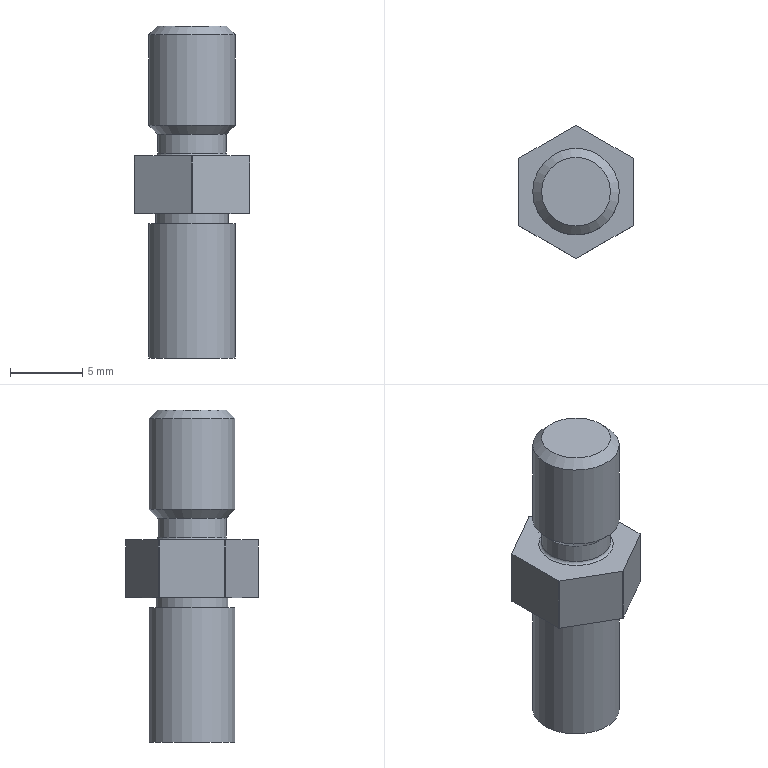Part | NX | features BREP 1 | 1 solid | 27 faces | box 8 x 9.2 x 23 mm | volume 695.67 mm3 | plane 11 | cylinder 11 | cone 4 | torus 1 | commonest cylinder face diameters 9.2 x6 6 x2 2.459 x1 4.773 x1 5 x1
STEP:
#1=CARTESIAN_POINT('',(-0.03277,4.6,-9.));
#2=VERTEX_POINT('',#1);
#3=CARTESIAN_POINT('',(-0.03277,4.6,-13.));
#4=VERTEX_POINT('',#3);
#5=CARTESIAN_POINT('',(-0.03277,4.6,-23.));
#6=DIRECTION('',(0.,0.,-1.));
#7=VECTOR('',#6,1000.);
#8=LINE('',#5,#7);
#9=EDGE_CURVE('',#2,#4,#8,.T.);
#10=ORIENTED_EDGE('',*,*,#9,.T.);
#11=CARTESIAN_POINT('',(-3.967,2.328,-13.));
#12=VERTEX_POINT('',#11);
#13=CARTESIAN_POINT('',(0.,4.619,-13.));
#14=DIRECTION('',(-0.866,-0.5,0.));
#15=VECTOR('',#14,1000.);
#16=LINE('',#13,#15);
#17=EDGE_CURVE('',#4,#12,#16,.T.);
#18=ORIENTED_EDGE('',*,*,#17,.T.);
#19=CARTESIAN_POINT('',(-3.967,2.328,-9.));
#20=VERTEX_POINT('',#19);
#21=CARTESIAN_POINT('',(-3.967,2.328,-23.));
#22=DIRECTION('',(0.,0.,-1.));
#23=VECTOR('',#22,1000.);
#24=LINE('',#21,#23);
#25=EDGE_CURVE('',#20,#12,#24,.T.);
#26=ORIENTED_EDGE('',*,*,#25,.F.);
#27=CARTESIAN_POINT('',(0.,4.619,-9.));
#28=DIRECTION('',(-0.866,-0.5,0.));
#29=VECTOR('',#28,1000.);
#30=LINE('',#27,#29);
#31=EDGE_CURVE('',#2,#20,#30,.T.);
#32=ORIENTED_EDGE('',*,*,#31,.F.);
#33=EDGE_LOOP('',(#10,#18,#26,#32));
#34=FACE_BOUND('',#33,.T.);
#35=CARTESIAN_POINT('',(0.,4.619,-13.));
#36=DIRECTION('',(-0.5,0.866,0.));
#37=DIRECTION('',(-0.866,-0.5,0.));
#38=AXIS2_PLACEMENT_3D('',#35,#36,#37);
#39=PLANE('',#38);
#40=ADVANCED_FACE('',(#34),#39,.T.);
#41=CARTESIAN_POINT('',(3.967,2.328,-9.));
#42=VERTEX_POINT('',#41);
#43=CARTESIAN_POINT('',(3.967,2.328,-13.));
#44=VERTEX_POINT('',#43);
#45=CARTESIAN_POINT('',(3.967,2.328,-23.));
#46=DIRECTION('',(0.,0.,-1.));
#47=VECTOR('',#46,1000.);
#48=LINE('',#45,#47);
#49=EDGE_CURVE('',#42,#44,#48,.T.);
#50=ORIENTED_EDGE('',*,*,#49,.T.);
#51=CARTESIAN_POINT('',(0.03277,4.6,-13.));
#52=VERTEX_POINT('',#51);
#53=CARTESIAN_POINT('',(4.,2.309,-13.));
#54=DIRECTION('',(-0.866,0.5,0.));
#55=VECTOR('',#54,1000.);
#56=LINE('',#53,#55);
#57=EDGE_CURVE('',#44,#52,#56,.T.);
#58=ORIENTED_EDGE('',*,*,#57,.T.);
#59=CARTESIAN_POINT('',(0.03277,4.6,-9.));
#60=VERTEX_POINT('',#59);
#61=CARTESIAN_POINT('',(0.03277,4.6,-23.));
#62=DIRECTION('',(0.,0.,-1.));
#63=VECTOR('',#62,1000.);
#64=LINE('',#61,#63);
#65=EDGE_CURVE('',#60,#52,#64,.T.);
#66=ORIENTED_EDGE('',*,*,#65,.F.);
#67=CARTESIAN_POINT('',(4.,2.309,-9.));
#68=DIRECTION('',(-0.866,0.5,0.));
#69=VECTOR('',#68,1000.);
#70=LINE('',#67,#69);
#71=EDGE_CURVE('',#42,#60,#70,.T.);
#72=ORIENTED_EDGE('',*,*,#71,.F.);
#73=EDGE_LOOP('',(#50,#58,#66,#72));
#74=FACE_BOUND('',#73,.T.);
#75=CARTESIAN_POINT('',(4.,2.309,-13.));
#76=DIRECTION('',(0.5,0.866,0.));
#77=DIRECTION('',(-0.866,0.5,0.));
#78=AXIS2_PLACEMENT_3D('',#75,#76,#77);
#79=PLANE('',#78);
#80=ADVANCED_FACE('',(#74),#79,.T.);
#81=CARTESIAN_POINT('',(4.,-2.272,-9.));
#82=VERTEX_POINT('',#81);
#83=CARTESIAN_POINT('',(4.,-2.272,-13.));
#84=VERTEX_POINT('',#83);
#85=CARTESIAN_POINT('',(4.,-2.272,-23.));
#86=DIRECTION('',(0.,0.,-1.));
#87=VECTOR('',#86,1000.);
#88=LINE('',#85,#87);
#89=EDGE_CURVE('',#82,#84,#88,.T.);
#90=ORIENTED_EDGE('',*,*,#89,.T.);
#91=CARTESIAN_POINT('',(4.,2.272,-13.));
#92=VERTEX_POINT('',#91);
#93=CARTESIAN_POINT('',(4.,-2.309,-13.));
#94=DIRECTION('',(0.,1.,0.));
#95=VECTOR('',#94,1000.);
#96=LINE('',#93,#95);
#97=EDGE_CURVE('',#84,#92,#96,.T.);
#98=ORIENTED_EDGE('',*,*,#97,.T.);
#99=CARTESIAN_POINT('',(4.,2.272,-9.));
#100=VERTEX_POINT('',#99);
#101=CARTESIAN_POINT('',(4.,2.272,-23.));
#102=DIRECTION('',(0.,0.,-1.));
#103=VECTOR('',#102,1000.);
#104=LINE('',#101,#103);
#105=EDGE_CURVE('',#100,#92,#104,.T.);
#106=ORIENTED_EDGE('',*,*,#105,.F.);
#107=CARTESIAN_POINT('',(4.,-2.309,-9.));
#108=DIRECTION('',(0.,1.,0.));
#109=VECTOR('',#108,1000.);
#110=LINE('',#107,#109);
#111=EDGE_CURVE('',#82,#100,#110,.T.);
#112=ORIENTED_EDGE('',*,*,#111,.F.);
#113=EDGE_LOOP('',(#90,#98,#106,#112));
#114=FACE_BOUND('',#113,.T.);
#115=CARTESIAN_POINT('',(4.,-2.309,-13.));
#116=DIRECTION('',(1.,0.,0.));
#117=DIRECTION('',(0.,0.,-1.));
#118=AXIS2_PLACEMENT_3D('',#115,#116,#117);
#119=PLANE('',#118);
#120=ADVANCED_FACE('',(#114),#119,.T.);
#121=ORIENTED_EDGE('',*,*,#49,.F.);
#122=CARTESIAN_POINT('',(0.,0.,-9.));
#123=DIRECTION('',(0.,0.,-1.));
#124=DIRECTION('',(-1.,0.,0.));
#125=AXIS2_PLACEMENT_3D('',#122,#123,#124);
#126=CIRCLE('',#125,4.6);
#127=EDGE_CURVE('',#42,#100,#126,.T.);
#128=ORIENTED_EDGE('',*,*,#127,.T.);
#129=ORIENTED_EDGE('',*,*,#105,.T.);
#130=CARTESIAN_POINT('',(0.,0.,-13.));
#131=DIRECTION('',(0.,0.,-1.));
#132=DIRECTION('',(-1.,0.,0.));
#133=AXIS2_PLACEMENT_3D('',#130,#131,#132);
#134=CIRCLE('',#133,4.6);
#135=EDGE_CURVE('',#44,#92,#134,.T.);
#136=ORIENTED_EDGE('',*,*,#135,.F.);
#137=EDGE_LOOP('',(#121,#128,#129,#136));
#138=FACE_BOUND('',#137,.T.);
#139=CARTESIAN_POINT('',(0.,0.,-23.));
#140=DIRECTION('',(0.,0.,1.));
#141=DIRECTION('',(-1.,0.,0.));
#142=AXIS2_PLACEMENT_3D('',#139,#140,#141);
#143=CYLINDRICAL_SURFACE('',#142,4.6);
#144=ADVANCED_FACE('',(#138),#143,.T.);
#145=ORIENTED_EDGE('',*,*,#65,.T.);
#146=CARTESIAN_POINT('',(0.,0.,-13.));
#147=DIRECTION('',(0.,0.,-1.));
#148=DIRECTION('',(-1.,0.,0.));
#149=AXIS2_PLACEMENT_3D('',#146,#147,#148);
#150=CIRCLE('',#149,4.6);
#151=EDGE_CURVE('',#4,#52,#150,.T.);
#152=ORIENTED_EDGE('',*,*,#151,.F.);
#153=ORIENTED_EDGE('',*,*,#9,.F.);
#154=CARTESIAN_POINT('',(0.,0.,-9.));
#155=DIRECTION('',(0.,0.,-1.));
#156=DIRECTION('',(-1.,0.,0.));
#157=AXIS2_PLACEMENT_3D('',#154,#155,#156);
#158=CIRCLE('',#157,4.6);
#159=EDGE_CURVE('',#2,#60,#158,.T.);
#160=ORIENTED_EDGE('',*,*,#159,.T.);
#161=EDGE_LOOP('',(#145,#152,#153,#160));
#162=FACE_BOUND('',#161,.T.);
#163=CARTESIAN_POINT('',(0.,0.,-23.));
#164=DIRECTION('',(0.,0.,1.));
#165=DIRECTION('',(-1.,0.,0.));
#166=AXIS2_PLACEMENT_3D('',#163,#164,#165);
#167=CYLINDRICAL_SURFACE('',#166,4.6);
#168=ADVANCED_FACE('',(#162),#167,.T.);
#169=ORIENTED_EDGE('',*,*,#89,.F.);
#170=CARTESIAN_POINT('',(3.967,-2.328,-9.));
#171=VERTEX_POINT('',#170);
#172=CARTESIAN_POINT('',(0.,0.,-9.));
#173=DIRECTION('',(0.,0.,-1.));
#174=DIRECTION('',(-1.,0.,0.));
#175=AXIS2_PLACEMENT_3D('',#172,#173,#174);
#176=CIRCLE('',#175,4.6);
#177=EDGE_CURVE('',#82,#171,#176,.T.);
#178=ORIENTED_EDGE('',*,*,#177,.T.);
#179=CARTESIAN_POINT('',(3.967,-2.328,-13.));
#180=VERTEX_POINT('',#179);
#181=CARTESIAN_POINT('',(3.967,-2.328,-23.));
#182=DIRECTION('',(0.,0.,-1.));
#183=VECTOR('',#182,1000.);
#184=LINE('',#181,#183);
#185=EDGE_CURVE('',#171,#180,#184,.T.);
#186=ORIENTED_EDGE('',*,*,#185,.T.);
#187=CARTESIAN_POINT('',(0.,0.,-13.));
#188=DIRECTION('',(0.,0.,-1.));
#189=DIRECTION('',(-1.,0.,0.));
#190=AXIS2_PLACEMENT_3D('',#187,#188,#189);
#191=CIRCLE('',#190,4.6);
#192=EDGE_CURVE('',#84,#180,#191,.T.);
#193=ORIENTED_EDGE('',*,*,#192,.F.);
#194=EDGE_LOOP('',(#169,#178,#186,#193));
#195=FACE_BOUND('',#194,.T.);
#196=CARTESIAN_POINT('',(0.,0.,-23.));
#197=DIRECTION('',(0.,0.,1.));
#198=DIRECTION('',(-1.,0.,0.));
#199=AXIS2_PLACEMENT_3D('',#196,#197,#198);
#200=CYLINDRICAL_SURFACE('',#199,4.6);
#201=ADVANCED_FACE('',(#195),#200,.T.);
#202=CARTESIAN_POINT('',(0.03277,-4.6,-9.));
#203=VERTEX_POINT('',#202);
#204=CARTESIAN_POINT('',(0.03277,-4.6,-13.));
#205=VERTEX_POINT('',#204);
#206=CARTESIAN_POINT('',(0.03277,-4.6,-23.));
#207=DIRECTION('',(0.,0.,-1.));
#208=VECTOR('',#207,1000.);
#209=LINE('',#206,#208);
#210=EDGE_CURVE('',#203,#205,#209,.T.);
#211=ORIENTED_EDGE('',*,*,#210,.F.);
#212=CARTESIAN_POINT('',(-0.03277,-4.6,-9.));
#213=VERTEX_POINT('',#212);
#214=CARTESIAN_POINT('',(0.,0.,-9.));
#215=DIRECTION('',(0.,0.,-1.));
#216=DIRECTION('',(-1.,0.,0.));
#217=AXIS2_PLACEMENT_3D('',#214,#215,#216);
#218=CIRCLE('',#217,4.6);
#219=EDGE_CURVE('',#203,#213,#218,.T.);
#220=ORIENTED_EDGE('',*,*,#219,.T.);
#221=CARTESIAN_POINT('',(-0.03277,-4.6,-13.));
#222=VERTEX_POINT('',#221);
#223=CARTESIAN_POINT('',(-0.03277,-4.6,-23.));
#224=DIRECTION('',(0.,0.,-1.));
#225=VECTOR('',#224,1000.);
#226=LINE('',#223,#225);
#227=EDGE_CURVE('',#213,#222,#226,.T.);
#228=ORIENTED_EDGE('',*,*,#227,.T.);
#229=CARTESIAN_POINT('',(0.,0.,-13.));
#230=DIRECTION('',(0.,0.,-1.));
#231=DIRECTION('',(-1.,0.,0.));
#232=AXIS2_PLACEMENT_3D('',#229,#230,#231);
#233=CIRCLE('',#232,4.6);
#234=EDGE_CURVE('',#205,#222,#233,.T.);
#235=ORIENTED_EDGE('',*,*,#234,.F.);
#236=EDGE_LOOP('',(#211,#220,#228,#235));
#237=FACE_BOUND('',#236,.T.);
#238=CARTESIAN_POINT('',(0.,0.,-23.));
#239=DIRECTION('',(0.,0.,1.));
#240=DIRECTION('',(-1.,0.,0.));
#241=AXIS2_PLACEMENT_3D('',#238,#239,#240);
#242=CYLINDRICAL_SURFACE('',#241,4.6);
#243=ADVANCED_FACE('',(#237),#242,.T.);
#244=CARTESIAN_POINT('',(-1.23,0.,-16.));
#245=VERTEX_POINT('',#244);
#246=CARTESIAN_POINT('',(0.,0.,-16.));
#247=DIRECTION('',(0.,0.,-1.));
#248=DIRECTION('',(-1.,0.,0.));
#249=AXIS2_PLACEMENT_3D('',#246,#247,#248);
#250=CIRCLE('',#249,1.23);
#251=EDGE_CURVE('',#245,#245,#250,.T.);
#252=ORIENTED_EDGE('',*,*,#251,.T.);
#253=EDGE_LOOP('',(#252));
#254=FACE_BOUND('',#253,.T.);
#255=CARTESIAN_POINT('',(0.,0.,-15.));
#256=VERTEX_POINT('',#255);
#257=VERTEX_LOOP('',#256);
#258=FACE_BOUND('',#257,.T.);
#259=CARTESIAN_POINT('',(0.,0.,-16.));
#260=DIRECTION('',(0.,0.,-1.));
#261=DIRECTION('',(-1.,0.,0.));
#262=AXIS2_PLACEMENT_3D('',#259,#260,#261);
#263=CONICAL_SURFACE('',#262,1.23,0.888);
#264=ADVANCED_FACE('',(#254,#258),#263,.F.);
#265=CARTESIAN_POINT('',(-1.23,0.,-22.73));
#266=VERTEX_POINT('',#265);
#267=CARTESIAN_POINT('',(0.,0.,-22.73));
#268=DIRECTION('',(0.,0.,-1.));
#269=DIRECTION('',(-1.,0.,0.));
#270=AXIS2_PLACEMENT_3D('',#267,#268,#269);
#271=CIRCLE('',#270,1.23);
#272=EDGE_CURVE('',#266,#266,#271,.T.);
#273=ORIENTED_EDGE('',*,*,#272,.T.);
#274=EDGE_LOOP('',(#273));
#275=FACE_BOUND('',#274,.T.);
#276=ORIENTED_EDGE('',*,*,#251,.F.);
#277=EDGE_LOOP('',(#276));
#278=FACE_BOUND('',#277,.T.);
#279=CARTESIAN_POINT('',(0.,0.,-23.));
#280=DIRECTION('',(0.,0.,1.));
#281=DIRECTION('',(-1.,0.,0.));
#282=AXIS2_PLACEMENT_3D('',#279,#280,#281);
#283=CYLINDRICAL_SURFACE('',#282,1.23);
#284=ADVANCED_FACE('',(#275,#278),#283,.F.);
#285=CARTESIAN_POINT('',(-1.5,0.,-23.));
#286=VERTEX_POINT('',#285);
#287=CARTESIAN_POINT('',(0.,0.,-23.));
#288=DIRECTION('',(0.,0.,-1.));
#289=DIRECTION('',(-1.,0.,0.));
#290=AXIS2_PLACEMENT_3D('',#287,#288,#289);
#291=CIRCLE('',#290,1.5);
#292=EDGE_CURVE('',#286,#286,#291,.T.);
#293=ORIENTED_EDGE('',*,*,#292,.T.);
#294=EDGE_LOOP('',(#293));
#295=FACE_BOUND('',#294,.T.);
#296=ORIENTED_EDGE('',*,*,#272,.F.);
#297=EDGE_LOOP('',(#296));
#298=FACE_BOUND('',#297,.T.);
#299=CARTESIAN_POINT('',(0.,0.,-23.));
#300=DIRECTION('',(0.,0.,-1.));
#301=DIRECTION('',(-1.,0.,0.));
#302=AXIS2_PLACEMENT_3D('',#299,#300,#301);
#303=CONICAL_SURFACE('',#302,1.5,0.7854);
#304=ADVANCED_FACE('',(#295,#298),#303,.F.);
#305=CARTESIAN_POINT('',(-3.,0.,-23.));
#306=VERTEX_POINT('',#305);
#307=CARTESIAN_POINT('',(0.,0.,-23.));
#308=DIRECTION('',(0.,0.,-1.));
#309=DIRECTION('',(-1.,0.,0.));
#310=AXIS2_PLACEMENT_3D('',#307,#308,#309);
#311=CIRCLE('',#310,3.);
#312=EDGE_CURVE('',#306,#306,#311,.T.);
#313=ORIENTED_EDGE('',*,*,#312,.T.);
#314=EDGE_LOOP('',(#313));
#315=FACE_BOUND('',#314,.T.);
#316=ORIENTED_EDGE('',*,*,#292,.F.);
#317=EDGE_LOOP('',(#316));
#318=FACE_BOUND('',#317,.T.);
#319=CARTESIAN_POINT('',(0.,3.,-23.));
#320=DIRECTION('',(0.,0.,1.));
#321=DIRECTION('',(1.,0.,0.));
#322=AXIS2_PLACEMENT_3D('',#319,#320,#321);
#323=PLANE('',#322);
#324=ADVANCED_FACE('',(#315,#318),#323,.F.);
#325=CARTESIAN_POINT('',(-3.,0.,-13.7));
#326=VERTEX_POINT('',#325);
#327=CARTESIAN_POINT('',(0.,0.,-13.7));
#328=DIRECTION('',(0.,0.,-1.));
#329=DIRECTION('',(-1.,0.,0.));
#330=AXIS2_PLACEMENT_3D('',#327,#328,#329);
#331=CIRCLE('',#330,3.);
#332=EDGE_CURVE('',#326,#326,#331,.T.);
#333=ORIENTED_EDGE('',*,*,#332,.T.);
#334=EDGE_LOOP('',(#333));
#335=FACE_BOUND('',#334,.T.);
#336=ORIENTED_EDGE('',*,*,#312,.F.);
#337=EDGE_LOOP('',(#336));
#338=FACE_BOUND('',#337,.T.);
#339=CARTESIAN_POINT('',(0.,0.,-23.));
#340=DIRECTION('',(0.,0.,1.));
#341=DIRECTION('',(-1.,0.,0.));
#342=AXIS2_PLACEMENT_3D('',#339,#340,#341);
#343=CYLINDRICAL_SURFACE('',#342,3.);
#344=ADVANCED_FACE('',(#335,#338),#343,.T.);
#345=CARTESIAN_POINT('',(-2.5,0.,-13.7));
#346=VERTEX_POINT('',#345);
#347=CARTESIAN_POINT('',(0.,0.,-13.7));
#348=DIRECTION('',(0.,0.,-1.));
#349=DIRECTION('',(-1.,0.,0.));
#350=AXIS2_PLACEMENT_3D('',#347,#348,#349);
#351=CIRCLE('',#350,2.5);
#352=EDGE_CURVE('',#346,#346,#351,.T.);
#353=ORIENTED_EDGE('',*,*,#352,.T.);
#354=EDGE_LOOP('',(#353));
#355=FACE_BOUND('',#354,.T.);
#356=ORIENTED_EDGE('',*,*,#332,.F.);
#357=EDGE_LOOP('',(#356));
#358=FACE_BOUND('',#357,.T.);
#359=CARTESIAN_POINT('',(0.,2.5,-13.7));
#360=DIRECTION('',(0.,0.,-1.));
#361=DIRECTION('',(-1.,0.,0.));
#362=AXIS2_PLACEMENT_3D('',#359,#360,#361);
#363=PLANE('',#362);
#364=ADVANCED_FACE('',(#355,#358),#363,.F.);
#365=CARTESIAN_POINT('',(-2.5,0.,-13.));
#366=VERTEX_POINT('',#365);
#367=CARTESIAN_POINT('',(0.,0.,-13.));
#368=DIRECTION('',(0.,0.,-1.));
#369=DIRECTION('',(-1.,0.,0.));
#370=AXIS2_PLACEMENT_3D('',#367,#368,#369);
#371=CIRCLE('',#370,2.5);
#372=EDGE_CURVE('',#366,#366,#371,.T.);
#373=ORIENTED_EDGE('',*,*,#372,.T.);
#374=EDGE_LOOP('',(#373));
#375=FACE_BOUND('',#374,.T.);
#376=ORIENTED_EDGE('',*,*,#352,.F.);
#377=EDGE_LOOP('',(#376));
#378=FACE_BOUND('',#377,.T.);
#379=CARTESIAN_POINT('',(0.,0.,-23.));
#380=DIRECTION('',(0.,0.,1.));
#381=DIRECTION('',(-1.,0.,0.));
#382=AXIS2_PLACEMENT_3D('',#379,#380,#381);
#383=CYLINDRICAL_SURFACE('',#382,2.5);
#384=ADVANCED_FACE('',(#375,#378),#383,.T.);
#385=CARTESIAN_POINT('',(-3.967,-2.328,-9.));
#386=VERTEX_POINT('',#385);
#387=CARTESIAN_POINT('',(-3.967,-2.328,-13.));
#388=VERTEX_POINT('',#387);
#389=CARTESIAN_POINT('',(-3.967,-2.328,-23.));
#390=DIRECTION('',(0.,0.,-1.));
#391=VECTOR('',#390,1000.);
#392=LINE('',#389,#391);
#393=EDGE_CURVE('',#386,#388,#392,.T.);
#394=ORIENTED_EDGE('',*,*,#393,.F.);
#395=CARTESIAN_POINT('',(-4.,-2.272,-9.));
#396=VERTEX_POINT('',#395);
#397=CARTESIAN_POINT('',(0.,0.,-9.));
#398=DIRECTION('',(0.,0.,-1.));
#399=DIRECTION('',(-1.,0.,0.));
#400=AXIS2_PLACEMENT_3D('',#397,#398,#399);
#401=CIRCLE('',#400,4.6);
#402=EDGE_CURVE('',#386,#396,#401,.T.);
#403=ORIENTED_EDGE('',*,*,#402,.T.);
#404=CARTESIAN_POINT('',(-4.,-2.272,-13.));
#405=VERTEX_POINT('',#404);
#406=CARTESIAN_POINT('',(-4.,-2.272,-23.));
#407=DIRECTION('',(0.,0.,-1.));
#408=VECTOR('',#407,1000.);
#409=LINE('',#406,#408);
#410=EDGE_CURVE('',#396,#405,#409,.T.);
#411=ORIENTED_EDGE('',*,*,#410,.T.);
#412=CARTESIAN_POINT('',(0.,0.,-13.));
#413=DIRECTION('',(0.,0.,-1.));
#414=DIRECTION('',(-1.,0.,0.));
#415=AXIS2_PLACEMENT_3D('',#412,#413,#414);
#416=CIRCLE('',#415,4.6);
#417=EDGE_CURVE('',#388,#405,#416,.T.);
#418=ORIENTED_EDGE('',*,*,#417,.F.);
#419=EDGE_LOOP('',(#394,#403,#411,#418));
#420=FACE_BOUND('',#419,.T.);
#421=CARTESIAN_POINT('',(0.,0.,-23.));
#422=DIRECTION('',(0.,0.,1.));
#423=DIRECTION('',(-1.,0.,0.));
#424=AXIS2_PLACEMENT_3D('',#421,#422,#423);
#425=CYLINDRICAL_SURFACE('',#424,4.6);
#426=ADVANCED_FACE('',(#420),#425,.T.);
#427=ORIENTED_EDGE('',*,*,#17,.F.);
#428=ORIENTED_EDGE('',*,*,#151,.T.);
#429=ORIENTED_EDGE('',*,*,#57,.F.);
#430=ORIENTED_EDGE('',*,*,#135,.T.);
#431=ORIENTED_EDGE('',*,*,#97,.F.);
#432=ORIENTED_EDGE('',*,*,#192,.T.);
#433=CARTESIAN_POINT('',(0.,-4.619,-13.));
#434=DIRECTION('',(0.866,0.5,0.));
#435=VECTOR('',#434,1000.);
#436=LINE('',#433,#435);
#437=EDGE_CURVE('',#205,#180,#436,.T.);
#438=ORIENTED_EDGE('',*,*,#437,.F.);
#439=ORIENTED_EDGE('',*,*,#234,.T.);
#440=CARTESIAN_POINT('',(-4.,-2.309,-13.));
#441=DIRECTION('',(0.866,-0.5,0.));
#442=VECTOR('',#441,1000.);
#443=LINE('',#440,#442);
#444=EDGE_CURVE('',#388,#222,#443,.T.);
#445=ORIENTED_EDGE('',*,*,#444,.F.);
#446=ORIENTED_EDGE('',*,*,#417,.T.);
#447=CARTESIAN_POINT('',(-4.,2.272,-13.));
#448=VERTEX_POINT('',#447);
#449=CARTESIAN_POINT('',(-4.,2.309,-13.));
#450=DIRECTION('',(0.,-1.,0.));
#451=VECTOR('',#450,1000.);
#452=LINE('',#449,#451);
#453=EDGE_CURVE('',#448,#405,#452,.T.);
#454=ORIENTED_EDGE('',*,*,#453,.F.);
#455=CARTESIAN_POINT('',(0.,0.,-13.));
#456=DIRECTION('',(0.,0.,-1.));
#457=DIRECTION('',(-1.,0.,0.));
#458=AXIS2_PLACEMENT_3D('',#455,#456,#457);
#459=CIRCLE('',#458,4.6);
#460=EDGE_CURVE('',#448,#12,#459,.T.);
#461=ORIENTED_EDGE('',*,*,#460,.T.);
#462=EDGE_LOOP('',(#427,#428,#429,#430,#431,#432,#438,#439,#445,#446,#454,#461));
#463=FACE_BOUND('',#462,.T.);
#464=ORIENTED_EDGE('',*,*,#372,.F.);
#465=EDGE_LOOP('',(#464));
#466=FACE_BOUND('',#465,.T.);
#467=CARTESIAN_POINT('',(0.,4.6,-13.));
#468=DIRECTION('',(0.,0.,1.));
#469=DIRECTION('',(1.,0.,0.));
#470=AXIS2_PLACEMENT_3D('',#467,#468,#469);
#471=PLANE('',#470);
#472=ADVANCED_FACE('',(#463,#466),#471,.F.);
#473=CARTESIAN_POINT('',(-2.386,0.,0.));
#474=VERTEX_POINT('',#473);
#475=CARTESIAN_POINT('',(0.,0.,0.));
#476=DIRECTION('',(0.,0.,-1.));
#477=DIRECTION('',(-1.,0.,0.));
#478=AXIS2_PLACEMENT_3D('',#475,#476,#477);
#479=CIRCLE('',#478,2.386);
#480=EDGE_CURVE('',#474,#474,#479,.T.);
#481=ORIENTED_EDGE('',*,*,#480,.F.);
#482=EDGE_LOOP('',(#481));
#483=FACE_BOUND('',#482,.T.);
#484=CARTESIAN_POINT('',(0.,0.,0.));
#485=DIRECTION('',(0.,0.,-1.));
#486=DIRECTION('',(-1.,0.,0.));
#487=AXIS2_PLACEMENT_3D('',#484,#485,#486);
#488=PLANE('',#487);
#489=ADVANCED_FACE('',(#483),#488,.F.);
#490=ORIENTED_EDGE('',*,*,#480,.T.);
#491=EDGE_LOOP('',(#490));
#492=FACE_BOUND('',#491,.T.);
#493=CARTESIAN_POINT('',(-3.,0.,-0.6135));
#494=VERTEX_POINT('',#493);
#495=CARTESIAN_POINT('',(0.,0.,-0.6135));
#496=DIRECTION('',(0.,0.,-1.));
#497=DIRECTION('',(-1.,0.,0.));
#498=AXIS2_PLACEMENT_3D('',#495,#496,#497);
#499=CIRCLE('',#498,3.);
#500=EDGE_CURVE('',#494,#494,#499,.T.);
#501=ORIENTED_EDGE('',*,*,#500,.F.);
#502=EDGE_LOOP('',(#501));
#503=FACE_BOUND('',#502,.T.);
#504=CARTESIAN_POINT('',(0.,0.,0.));
#505=DIRECTION('',(0.,0.,-1.));
#506=DIRECTION('',(-1.,0.,0.));
#507=AXIS2_PLACEMENT_3D('',#504,#505,#506);
#508=CONICAL_SURFACE('',#507,2.386,0.7854);
#509=ADVANCED_FACE('',(#492,#503),#508,.T.);
#510=ORIENTED_EDGE('',*,*,#500,.T.);
#511=EDGE_LOOP('',(#510));
#512=FACE_BOUND('',#511,.T.);
#513=CARTESIAN_POINT('',(-3.,0.,-6.886));
#514=VERTEX_POINT('',#513);
#515=CARTESIAN_POINT('',(0.,0.,-6.886));
#516=DIRECTION('',(0.,0.,-1.));
#517=DIRECTION('',(-1.,0.,0.));
#518=AXIS2_PLACEMENT_3D('',#515,#516,#517);
#519=CIRCLE('',#518,3.);
#520=EDGE_CURVE('',#514,#514,#519,.T.);
#521=ORIENTED_EDGE('',*,*,#520,.F.);
#522=EDGE_LOOP('',(#521));
#523=FACE_BOUND('',#522,.T.);
#524=CARTESIAN_POINT('',(0.,0.,-23.));
#525=DIRECTION('',(0.,0.,1.));
#526=DIRECTION('',(-1.,0.,0.));
#527=AXIS2_PLACEMENT_3D('',#524,#525,#526);
#528=CYLINDRICAL_SURFACE('',#527,3.);
#529=ADVANCED_FACE('',(#512,#523),#528,.T.);
#530=ORIENTED_EDGE('',*,*,#520,.T.);
#531=EDGE_LOOP('',(#530));
#532=FACE_BOUND('',#531,.T.);
#533=CARTESIAN_POINT('',(-2.386,0.,-7.5));
#534=VERTEX_POINT('',#533);
#535=CARTESIAN_POINT('',(0.,0.,-7.5));
#536=DIRECTION('',(0.,0.,-1.));
#537=DIRECTION('',(-1.,0.,0.));
#538=AXIS2_PLACEMENT_3D('',#535,#536,#537);
#539=CIRCLE('',#538,2.386);
#540=EDGE_CURVE('',#534,#534,#539,.T.);
#541=ORIENTED_EDGE('',*,*,#540,.F.);
#542=EDGE_LOOP('',(#541));
#543=FACE_BOUND('',#542,.T.);
#544=CARTESIAN_POINT('',(0.,0.,-6.886));
#545=DIRECTION('',(0.,0.,1.));
#546=DIRECTION('',(1.,0.,0.));
#547=AXIS2_PLACEMENT_3D('',#544,#545,#546);
#548=CONICAL_SURFACE('',#547,3.,0.7854);
#549=ADVANCED_FACE('',(#532,#543),#548,.T.);
#550=ORIENTED_EDGE('',*,*,#540,.T.);
#551=EDGE_LOOP('',(#550));
#552=FACE_BOUND('',#551,.T.);
#553=CARTESIAN_POINT('',(-2.386,0.,-8.8));
#554=VERTEX_POINT('',#553);
#555=CARTESIAN_POINT('',(0.,0.,-8.8));
#556=DIRECTION('',(0.,0.,-1.));
#557=DIRECTION('',(-1.,0.,0.));
#558=AXIS2_PLACEMENT_3D('',#555,#556,#557);
#559=CIRCLE('',#558,2.386);
#560=EDGE_CURVE('',#554,#554,#559,.T.);
#561=ORIENTED_EDGE('',*,*,#560,.F.);
#562=EDGE_LOOP('',(#561));
#563=FACE_BOUND('',#562,.T.);
#564=CARTESIAN_POINT('',(0.,0.,-23.));
#565=DIRECTION('',(0.,0.,1.));
#566=DIRECTION('',(-1.,0.,0.));
#567=AXIS2_PLACEMENT_3D('',#564,#565,#566);
#568=CYLINDRICAL_SURFACE('',#567,2.386);
#569=ADVANCED_FACE('',(#552,#563),#568,.T.);
#570=ORIENTED_EDGE('',*,*,#560,.T.);
#571=EDGE_LOOP('',(#570));
#572=FACE_BOUND('',#571,.T.);
#573=CARTESIAN_POINT('',(-2.587,0.,-9.));
#574=VERTEX_POINT('',#573);
#575=CARTESIAN_POINT('',(0.,0.,-9.));
#576=DIRECTION('',(0.,0.,-1.));
#577=DIRECTION('',(-1.,0.,0.));
#578=AXIS2_PLACEMENT_3D('',#575,#576,#577);
#579=CIRCLE('',#578,2.587);
#580=EDGE_CURVE('',#574,#574,#579,.T.);
#581=ORIENTED_EDGE('',*,*,#580,.F.);
#582=EDGE_LOOP('',(#581));
#583=FACE_BOUND('',#582,.T.);
#584=CARTESIAN_POINT('',(0.,0.,-8.8));
#585=DIRECTION('',(0.,0.,-1.));
#586=DIRECTION('',(-1.,0.,0.));
#587=AXIS2_PLACEMENT_3D('',#584,#585,#586);
#588=TOROIDAL_SURFACE('',#587,2.587,0.2);
#589=ADVANCED_FACE('',(#572,#583),#588,.F.);
#590=ORIENTED_EDGE('',*,*,#25,.T.);
#591=ORIENTED_EDGE('',*,*,#460,.F.);
#592=CARTESIAN_POINT('',(-4.,2.272,-9.));
#593=VERTEX_POINT('',#592);
#594=CARTESIAN_POINT('',(-4.,2.272,-23.));
#595=DIRECTION('',(0.,0.,-1.));
#596=VECTOR('',#595,1000.);
#597=LINE('',#594,#596);
#598=EDGE_CURVE('',#593,#448,#597,.T.);
#599=ORIENTED_EDGE('',*,*,#598,.F.);
#600=CARTESIAN_POINT('',(0.,0.,-9.));
#601=DIRECTION('',(0.,0.,-1.));
#602=DIRECTION('',(-1.,0.,0.));
#603=AXIS2_PLACEMENT_3D('',#600,#601,#602);
#604=CIRCLE('',#603,4.6);
#605=EDGE_CURVE('',#593,#20,#604,.T.);
#606=ORIENTED_EDGE('',*,*,#605,.T.);
#607=EDGE_LOOP('',(#590,#591,#599,#606));
#608=FACE_BOUND('',#607,.T.);
#609=CARTESIAN_POINT('',(0.,0.,-23.));
#610=DIRECTION('',(0.,0.,1.));
#611=DIRECTION('',(-1.,0.,0.));
#612=AXIS2_PLACEMENT_3D('',#609,#610,#611);
#613=CYLINDRICAL_SURFACE('',#612,4.6);
#614=ADVANCED_FACE('',(#608),#613,.T.);
#615=ORIENTED_EDGE('',*,*,#580,.T.);
#616=EDGE_LOOP('',(#615));
#617=FACE_BOUND('',#616,.T.);
#618=ORIENTED_EDGE('',*,*,#159,.F.);
#619=ORIENTED_EDGE('',*,*,#31,.T.);
#620=ORIENTED_EDGE('',*,*,#605,.F.);
#621=CARTESIAN_POINT('',(-4.,2.309,-9.));
#622=DIRECTION('',(0.,-1.,0.));
#623=VECTOR('',#622,1000.);
#624=LINE('',#621,#623);
#625=EDGE_CURVE('',#593,#396,#624,.T.);
#626=ORIENTED_EDGE('',*,*,#625,.T.);
#627=ORIENTED_EDGE('',*,*,#402,.F.);
#628=CARTESIAN_POINT('',(-4.,-2.309,-9.));
#629=DIRECTION('',(0.866,-0.5,0.));
#630=VECTOR('',#629,1000.);
#631=LINE('',#628,#630);
#632=EDGE_CURVE('',#386,#213,#631,.T.);
#633=ORIENTED_EDGE('',*,*,#632,.T.);
#634=ORIENTED_EDGE('',*,*,#219,.F.);
#635=CARTESIAN_POINT('',(0.,-4.619,-9.));
#636=DIRECTION('',(0.866,0.5,0.));
#637=VECTOR('',#636,1000.);
#638=LINE('',#635,#637);
#639=EDGE_CURVE('',#203,#171,#638,.T.);
#640=ORIENTED_EDGE('',*,*,#639,.T.);
#641=ORIENTED_EDGE('',*,*,#177,.F.);
#642=ORIENTED_EDGE('',*,*,#111,.T.);
#643=ORIENTED_EDGE('',*,*,#127,.F.);
#644=ORIENTED_EDGE('',*,*,#71,.T.);
#645=EDGE_LOOP('',(#618,#619,#620,#626,#627,#633,#634,#640,#641,#642,#643,#644));
#646=FACE_BOUND('',#645,.T.);
#647=CARTESIAN_POINT('',(0.,2.587,-9.));
#648=DIRECTION('',(0.,0.,-1.));
#649=DIRECTION('',(-1.,0.,0.));
#650=AXIS2_PLACEMENT_3D('',#647,#648,#649);
#651=PLANE('',#650);
#652=ADVANCED_FACE('',(#617,#646),#651,.F.);
#653=ORIENTED_EDGE('',*,*,#598,.T.);
#654=ORIENTED_EDGE('',*,*,#453,.T.);
#655=ORIENTED_EDGE('',*,*,#410,.F.);
#656=ORIENTED_EDGE('',*,*,#625,.F.);
#657=EDGE_LOOP('',(#653,#654,#655,#656));
#658=FACE_BOUND('',#657,.T.);
#659=CARTESIAN_POINT('',(-4.,2.309,-13.));
#660=DIRECTION('',(-1.,0.,0.));
#661=DIRECTION('',(0.,0.,1.));
#662=AXIS2_PLACEMENT_3D('',#659,#660,#661);
#663=PLANE('',#662);
#664=ADVANCED_FACE('',(#658),#663,.T.);
#665=ORIENTED_EDGE('',*,*,#210,.T.);
#666=ORIENTED_EDGE('',*,*,#437,.T.);
#667=ORIENTED_EDGE('',*,*,#185,.F.);
#668=ORIENTED_EDGE('',*,*,#639,.F.);
#669=EDGE_LOOP('',(#665,#666,#667,#668));
#670=FACE_BOUND('',#669,.T.);
#671=CARTESIAN_POINT('',(0.,-4.619,-13.));
#672=DIRECTION('',(0.5,-0.866,0.));
#673=DIRECTION('',(0.866,0.5,0.));
#674=AXIS2_PLACEMENT_3D('',#671,#672,#673);
#675=PLANE('',#674);
#676=ADVANCED_FACE('',(#670),#675,.T.);
#677=ORIENTED_EDGE('',*,*,#393,.T.);
#678=ORIENTED_EDGE('',*,*,#444,.T.);
#679=ORIENTED_EDGE('',*,*,#227,.F.);
#680=ORIENTED_EDGE('',*,*,#632,.F.);
#681=EDGE_LOOP('',(#677,#678,#679,#680));
#682=FACE_BOUND('',#681,.T.);
#683=CARTESIAN_POINT('',(-4.,-2.309,-13.));
#684=DIRECTION('',(-0.5,-0.866,0.));
#685=DIRECTION('',(0.866,-0.5,0.));
#686=AXIS2_PLACEMENT_3D('',#683,#684,#685);
#687=PLANE('',#686);
#688=ADVANCED_FACE('',(#682),#687,.T.);
#689=CLOSED_SHELL('',(#40,#80,#120,#144,#168,#201,#243,#264,#284,#304,#324,#344,#364,#384,#426,#472,#489,#509,#529,#549,#569,#589,#614,#652,#664,#676,#688));
#690=MANIFOLD_SOLID_BREP('',#689);
#691=(LENGTH_UNIT()NAMED_UNIT(*)SI_UNIT(.MILLI.,.METRE.));
#692=UNCERTAINTY_MEASURE_WITH_UNIT(LENGTH_MEASURE(0.00001),#691,'','');
#693=(NAMED_UNIT(*)PLANE_ANGLE_UNIT()SI_UNIT($,.RADIAN.));
#694=(NAMED_UNIT(*)SI_UNIT($,.STERADIAN.)SOLID_ANGLE_UNIT());
#695=(GEOMETRIC_REPRESENTATION_CONTEXT(3)GLOBAL_UNCERTAINTY_ASSIGNED_CONTEXT((#692))GLOBAL_UNIT_ASSIGNED_CONTEXT((#691,#693,#694))REPRESENTATION_CONTEXT('',''));
#696=ADVANCED_BREP_SHAPE_REPRESENTATION('',(#690),#695);